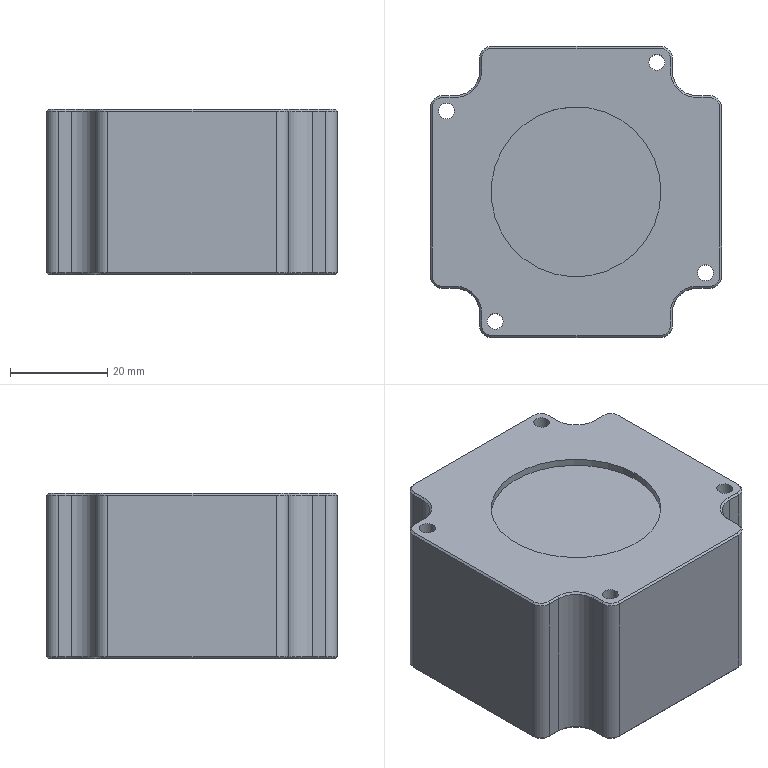Part | STEP file | 1 solid | 80 faces | box 60 x 60 x 34.1 mm | volume 106428 mm3 | plane 39 | cone 24 | cylinder 17 | commonest cylinder face diameters 5 x8 3.3 x4 10 x4 35 x1